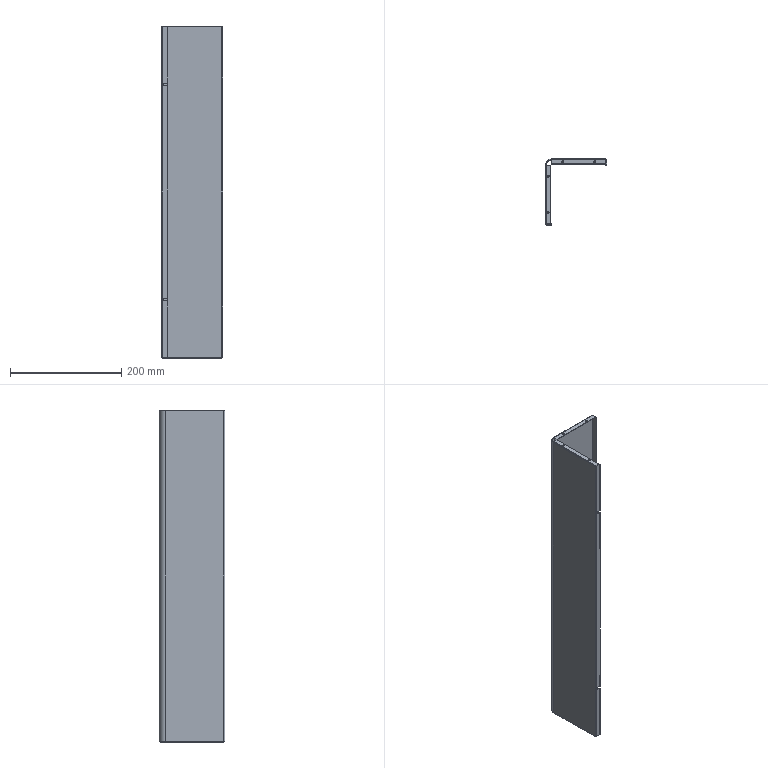Part | SolidWorks | features EdgeFlange 3, ICE 2, FlatPattern 1, HoleWzd 1, SMBaseFlange 1, SheetMetal 1 | 1 solid | 104 faces | box 110 x 118 x 598 mm | volume 147295 mm3 | plane 68 | cylinder 36 | commonest cylinder face diameters 3.3 x16 1 x6 3 x6 4.5 x6 20 x1 22 x1